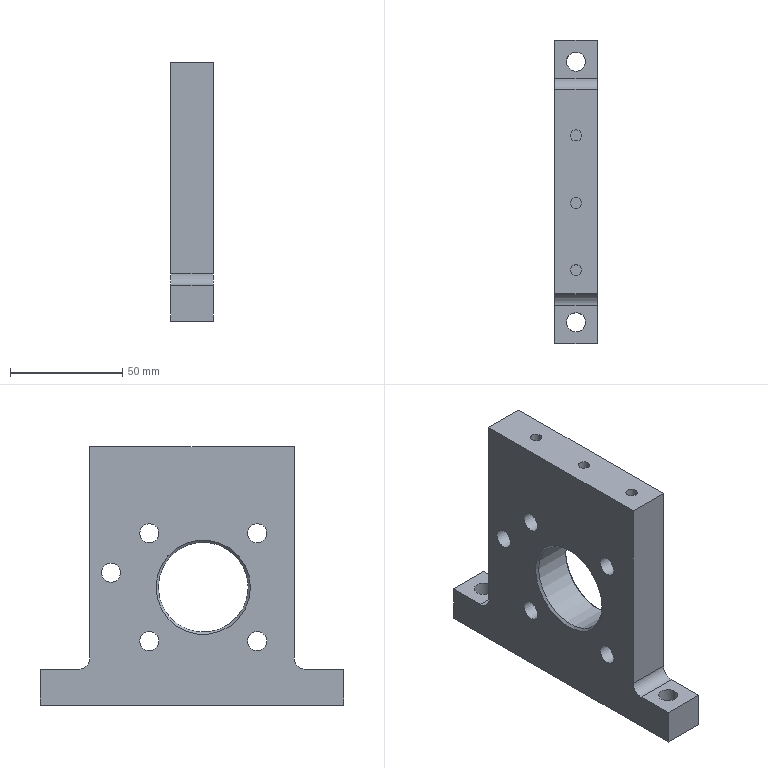Part | NX | 1 solid | 38 faces | box 19 x 135 x 115 mm | volume 176190 mm3 | cylinder 18 | plane 18 | cone 2 | commonest cylinder face diameters 8.5 x7 14 x5 5 x3 10 x2 40 x1
STEP:
#1=CARTESIAN_POINT('',(936.094,324.443,-201.3));
#2=VERTEX_POINT('',#1);
#3=CARTESIAN_POINT('',(936.094,317.443,-201.3));
#4=DIRECTION('',(-1.,0.,0.));
#5=DIRECTION('',(0.,1.,0.));
#6=AXIS2_PLACEMENT_3D('',#3,#4,#5);
#7=CIRCLE('',#6,7.);
#8=EDGE_CURVE('',#2,#2,#7,.T.);
#9=ORIENTED_EDGE('',*,*,#8,.F.);
#10=EDGE_LOOP('',(#9));
#11=FACE_BOUND('',#10,.T.);
#12=CARTESIAN_POINT('',(927.594,324.443,-201.3));
#13=VERTEX_POINT('',#12);
#14=CARTESIAN_POINT('',(927.594,317.443,-201.3));
#15=DIRECTION('',(-1.,0.,0.));
#16=DIRECTION('',(0.,1.,0.));
#17=AXIS2_PLACEMENT_3D('',#14,#15,#16);
#18=CIRCLE('',#17,7.);
#19=EDGE_CURVE('',#13,#13,#18,.T.);
#20=ORIENTED_EDGE('',*,*,#19,.T.);
#21=EDGE_LOOP('',(#20));
#22=FACE_BOUND('',#21,.T.);
#23=CARTESIAN_POINT('',(936.094,317.443,-201.3));
#24=DIRECTION('',(-1.,0.,0.));
#25=DIRECTION('',(0.,1.,0.));
#26=AXIS2_PLACEMENT_3D('',#23,#24,#25);
#27=CYLINDRICAL_SURFACE('',#26,7.);
#28=ADVANCED_FACE('',(#11,#22),#27,.F.);
#29=CARTESIAN_POINT('',(927.594,321.693,-201.3));
#30=VERTEX_POINT('',#29);
#31=CARTESIAN_POINT('',(927.594,317.443,-201.3));
#32=DIRECTION('',(1.,0.,0.));
#33=DIRECTION('',(0.,1.,0.));
#34=AXIS2_PLACEMENT_3D('',#31,#32,#33);
#35=CIRCLE('',#34,4.25);
#36=EDGE_CURVE('',#30,#30,#35,.T.);
#37=ORIENTED_EDGE('',*,*,#36,.F.);
#38=EDGE_LOOP('',(#37));
#39=FACE_BOUND('',#38,.T.);
#40=ORIENTED_EDGE('',*,*,#19,.F.);
#41=EDGE_LOOP('',(#40));
#42=FACE_BOUND('',#41,.T.);
#43=CARTESIAN_POINT('',(927.594,317.443,-201.3));
#44=DIRECTION('',(-1.,0.,0.));
#45=DIRECTION('',(0.,1.,0.));
#46=AXIS2_PLACEMENT_3D('',#43,#44,#45);
#47=PLANE('',#46);
#48=ADVANCED_FACE('',(#39,#42),#47,.F.);
#49=CARTESIAN_POINT('',(917.094,313.193,-201.3));
#50=VERTEX_POINT('',#49);
#51=CARTESIAN_POINT('',(917.094,317.443,-201.3));
#52=DIRECTION('',(1.,0.,0.));
#53=DIRECTION('',(0.,-1.,0.));
#54=AXIS2_PLACEMENT_3D('',#51,#52,#53);
#55=CIRCLE('',#54,4.25);
#56=EDGE_CURVE('',#50,#50,#55,.T.);
#57=ORIENTED_EDGE('',*,*,#56,.F.);
#58=EDGE_LOOP('',(#57));
#59=FACE_BOUND('',#58,.T.);
#60=ORIENTED_EDGE('',*,*,#36,.T.);
#61=EDGE_LOOP('',(#60));
#62=FACE_BOUND('',#61,.T.);
#63=CARTESIAN_POINT('',(917.094,317.443,-201.3));
#64=DIRECTION('',(1.,0.,0.));
#65=DIRECTION('',(0.,-1.,0.));
#66=AXIS2_PLACEMENT_3D('',#63,#64,#65);
#67=CYLINDRICAL_SURFACE('',#66,4.25);
#68=ADVANCED_FACE('',(#59,#62),#67,.F.);
#69=CARTESIAN_POINT('',(926.594,335.193,-260.3));
#70=VERTEX_POINT('',#69);
#71=CARTESIAN_POINT('',(926.594,339.443,-260.3));
#72=DIRECTION('',(0.,0.,1.));
#73=DIRECTION('',(0.,-1.,0.));
#74=AXIS2_PLACEMENT_3D('',#71,#72,#73);
#75=CIRCLE('',#74,4.25);
#76=EDGE_CURVE('',#70,#70,#75,.T.);
#77=ORIENTED_EDGE('',*,*,#76,.F.);
#78=EDGE_LOOP('',(#77));
#79=FACE_BOUND('',#78,.T.);
#80=CARTESIAN_POINT('',(930.844,339.443,-244.3));
#81=VERTEX_POINT('',#80);
#82=CARTESIAN_POINT('',(926.594,339.443,-244.3));
#83=DIRECTION('',(0.,0.,-1.));
#84=DIRECTION('',(1.,0.,0.));
#85=AXIS2_PLACEMENT_3D('',#82,#83,#84);
#86=CIRCLE('',#85,4.25);
#87=EDGE_CURVE('',#81,#81,#86,.T.);
#88=ORIENTED_EDGE('',*,*,#87,.F.);
#89=EDGE_LOOP('',(#88));
#90=FACE_BOUND('',#89,.T.);
#91=CARTESIAN_POINT('',(926.594,339.443,-244.3));
#92=DIRECTION('',(0.,0.,-1.));
#93=DIRECTION('',(-1.,0.,0.));
#94=AXIS2_PLACEMENT_3D('',#91,#92,#93);
#95=CYLINDRICAL_SURFACE('',#94,4.25);
#96=ADVANCED_FACE('',(#79,#90),#95,.F.);
#97=CARTESIAN_POINT('',(926.594,219.193,-260.3));
#98=VERTEX_POINT('',#97);
#99=CARTESIAN_POINT('',(926.594,223.443,-260.3));
#100=DIRECTION('',(0.,0.,1.));
#101=DIRECTION('',(0.,-1.,0.));
#102=AXIS2_PLACEMENT_3D('',#99,#100,#101);
#103=CIRCLE('',#102,4.25);
#104=EDGE_CURVE('',#98,#98,#103,.T.);
#105=ORIENTED_EDGE('',*,*,#104,.F.);
#106=EDGE_LOOP('',(#105));
#107=FACE_BOUND('',#106,.T.);
#108=CARTESIAN_POINT('',(922.344,223.443,-244.3));
#109=VERTEX_POINT('',#108);
#110=CARTESIAN_POINT('',(926.594,223.443,-244.3));
#111=DIRECTION('',(0.,0.,-1.));
#112=DIRECTION('',(-1.,0.,0.));
#113=AXIS2_PLACEMENT_3D('',#110,#111,#112);
#114=CIRCLE('',#113,4.25);
#115=EDGE_CURVE('',#109,#109,#114,.T.);
#116=ORIENTED_EDGE('',*,*,#115,.F.);
#117=EDGE_LOOP('',(#116));
#118=FACE_BOUND('',#117,.T.);
#119=CARTESIAN_POINT('',(926.594,223.443,-244.3));
#120=DIRECTION('',(0.,0.,-1.));
#121=DIRECTION('',(-1.,0.,0.));
#122=AXIS2_PLACEMENT_3D('',#119,#120,#121);
#123=CYLINDRICAL_SURFACE('',#122,4.25);
#124=ADVANCED_FACE('',(#107,#118),#123,.F.);
#125=CARTESIAN_POINT('',(924.094,276.443,-160.3));
#126=VERTEX_POINT('',#125);
#127=CARTESIAN_POINT('',(926.594,276.443,-160.3));
#128=DIRECTION('',(0.,0.,1.));
#129=DIRECTION('',(-1.,0.,0.));
#130=AXIS2_PLACEMENT_3D('',#127,#128,#129);
#131=CIRCLE('',#130,2.5);
#132=EDGE_CURVE('',#126,#126,#131,.T.);
#133=ORIENTED_EDGE('',*,*,#132,.T.);
#134=EDGE_LOOP('',(#133));
#135=FACE_BOUND('',#134,.T.);
#136=CARTESIAN_POINT('',(926.594,281.943,-160.3));
#137=DIRECTION('',(0.,0.,-1.));
#138=DIRECTION('',(0.,1.,0.));
#139=AXIS2_PLACEMENT_3D('',#136,#137,#138);
#140=PLANE('',#139);
#141=ADVANCED_FACE('',(#135),#140,.F.);
#142=ORIENTED_EDGE('',*,*,#132,.F.);
#143=EDGE_LOOP('',(#142));
#144=FACE_BOUND('',#143,.T.);
#145=CARTESIAN_POINT('',(924.094,276.443,-145.3));
#146=VERTEX_POINT('',#145);
#147=CARTESIAN_POINT('',(926.594,276.443,-145.3));
#148=DIRECTION('',(0.,0.,1.));
#149=DIRECTION('',(-1.,0.,0.));
#150=AXIS2_PLACEMENT_3D('',#147,#148,#149);
#151=CIRCLE('',#150,2.5);
#152=EDGE_CURVE('',#146,#146,#151,.T.);
#153=ORIENTED_EDGE('',*,*,#152,.T.);
#154=EDGE_LOOP('',(#153));
#155=FACE_BOUND('',#154,.T.);
#156=CARTESIAN_POINT('',(926.594,276.443,-145.3));
#157=DIRECTION('',(0.,0.,-1.));
#158=DIRECTION('',(-1.,0.,0.));
#159=AXIS2_PLACEMENT_3D('',#156,#157,#158);
#160=CYLINDRICAL_SURFACE('',#159,2.5);
#161=ADVANCED_FACE('',(#144,#155),#160,.F.);
#162=CARTESIAN_POINT('',(935.094,256.443,-207.8));
#163=VERTEX_POINT('',#162);
#164=CARTESIAN_POINT('',(935.094,276.443,-207.8));
#165=DIRECTION('',(1.,0.,0.));
#166=DIRECTION('',(0.,-1.,0.));
#167=AXIS2_PLACEMENT_3D('',#164,#165,#166);
#168=CIRCLE('',#167,20.);
#169=EDGE_CURVE('',#163,#163,#168,.T.);
#170=ORIENTED_EDGE('',*,*,#169,.F.);
#171=EDGE_LOOP('',(#170));
#172=FACE_BOUND('',#171,.T.);
#173=CARTESIAN_POINT('',(936.094,255.443,-207.8));
#174=VERTEX_POINT('',#173);
#175=CARTESIAN_POINT('',(936.094,276.443,-207.8));
#176=DIRECTION('',(-1.,0.,0.));
#177=DIRECTION('',(0.,-1.,0.));
#178=AXIS2_PLACEMENT_3D('',#175,#176,#177);
#179=CIRCLE('',#178,21.);
#180=EDGE_CURVE('',#174,#174,#179,.T.);
#181=ORIENTED_EDGE('',*,*,#180,.F.);
#182=EDGE_LOOP('',(#181));
#183=FACE_BOUND('',#182,.T.);
#184=CARTESIAN_POINT('',(935.094,276.443,-207.8));
#185=DIRECTION('',(1.,0.,0.));
#186=DIRECTION('',(0.,-1.,0.));
#187=AXIS2_PLACEMENT_3D('',#184,#185,#186);
#188=CONICAL_SURFACE('',#187,20.,0.7854);
#189=ADVANCED_FACE('',(#172,#183),#188,.F.);
#190=CARTESIAN_POINT('',(927.594,252.443,-227.55));
#191=VERTEX_POINT('',#190);
#192=CARTESIAN_POINT('',(927.594,252.443,-231.8));
#193=DIRECTION('',(-1.,0.,0.));
#194=DIRECTION('',(0.,0.,1.));
#195=AXIS2_PLACEMENT_3D('',#192,#193,#194);
#196=CIRCLE('',#195,4.25);
#197=EDGE_CURVE('',#191,#191,#196,.T.);
#198=ORIENTED_EDGE('',*,*,#197,.T.);
#199=EDGE_LOOP('',(#198));
#200=FACE_BOUND('',#199,.T.);
#201=CARTESIAN_POINT('',(927.594,252.443,-224.8));
#202=VERTEX_POINT('',#201);
#203=CARTESIAN_POINT('',(927.594,252.443,-231.8));
#204=DIRECTION('',(1.,0.,0.));
#205=DIRECTION('',(0.,0.,1.));
#206=AXIS2_PLACEMENT_3D('',#203,#204,#205);
#207=CIRCLE('',#206,7.);
#208=EDGE_CURVE('',#202,#202,#207,.T.);
#209=ORIENTED_EDGE('',*,*,#208,.T.);
#210=EDGE_LOOP('',(#209));
#211=FACE_BOUND('',#210,.T.);
#212=CARTESIAN_POINT('',(927.594,317.443,-201.3));
#213=DIRECTION('',(-1.,0.,0.));
#214=DIRECTION('',(0.,1.,0.));
#215=AXIS2_PLACEMENT_3D('',#212,#213,#214);
#216=PLANE('',#215);
#217=ADVANCED_FACE('',(#200,#211),#216,.F.);
#218=CARTESIAN_POINT('',(918.094,296.443,-207.8));
#219=VERTEX_POINT('',#218);
#220=CARTESIAN_POINT('',(918.094,276.443,-207.8));
#221=DIRECTION('',(-1.,0.,0.));
#222=DIRECTION('',(0.,1.,0.));
#223=AXIS2_PLACEMENT_3D('',#220,#221,#222);
#224=CIRCLE('',#223,20.);
#225=EDGE_CURVE('',#219,#219,#224,.T.);
#226=ORIENTED_EDGE('',*,*,#225,.F.);
#227=EDGE_LOOP('',(#226));
#228=FACE_BOUND('',#227,.T.);
#229=CARTESIAN_POINT('',(917.094,297.443,-207.8));
#230=VERTEX_POINT('',#229);
#231=CARTESIAN_POINT('',(917.094,276.443,-207.8));
#232=DIRECTION('',(1.,0.,0.));
#233=DIRECTION('',(0.,1.,0.));
#234=AXIS2_PLACEMENT_3D('',#231,#232,#233);
#235=CIRCLE('',#234,21.);
#236=EDGE_CURVE('',#230,#230,#235,.T.);
#237=ORIENTED_EDGE('',*,*,#236,.F.);
#238=EDGE_LOOP('',(#237));
#239=FACE_BOUND('',#238,.T.);
#240=CARTESIAN_POINT('',(918.094,276.443,-207.8));
#241=DIRECTION('',(-1.,0.,0.));
#242=DIRECTION('',(0.,1.,0.));
#243=AXIS2_PLACEMENT_3D('',#240,#241,#242);
#244=CONICAL_SURFACE('',#243,20.,0.7854);
#245=ADVANCED_FACE('',(#228,#239),#244,.F.);
#246=CARTESIAN_POINT('',(917.094,235.943,-239.3));
#247=VERTEX_POINT('',#246);
#248=CARTESIAN_POINT('',(917.094,235.943,-145.3));
#249=VERTEX_POINT('',#248);
#250=CARTESIAN_POINT('',(917.094,235.943,-204.8));
#251=DIRECTION('',(0.,0.,1.));
#252=VECTOR('',#251,1000.);
#253=LINE('',#250,#252);
#254=EDGE_CURVE('',#247,#249,#253,.T.);
#255=ORIENTED_EDGE('',*,*,#254,.T.);
#256=CARTESIAN_POINT('',(917.094,326.943,-145.3));
#257=VERTEX_POINT('',#256);
#258=CARTESIAN_POINT('',(917.094,329.943,-145.3));
#259=DIRECTION('',(0.,1.,0.));
#260=VECTOR('',#259,1000.);
#261=LINE('',#258,#260);
#262=EDGE_CURVE('',#249,#257,#261,.T.);
#263=ORIENTED_EDGE('',*,*,#262,.T.);
#264=CARTESIAN_POINT('',(917.094,326.943,-239.3));
#265=VERTEX_POINT('',#264);
#266=CARTESIAN_POINT('',(917.094,326.943,-204.8));
#267=DIRECTION('',(0.,0.,-1.));
#268=VECTOR('',#267,1000.);
#269=LINE('',#266,#268);
#270=EDGE_CURVE('',#257,#265,#269,.T.);
#271=ORIENTED_EDGE('',*,*,#270,.T.);
#272=CARTESIAN_POINT('',(917.094,331.943,-244.3));
#273=VERTEX_POINT('',#272);
#274=CARTESIAN_POINT('',(917.094,331.943,-239.3));
#275=DIRECTION('',(1.,0.,0.));
#276=DIRECTION('',(0.,1.,0.));
#277=AXIS2_PLACEMENT_3D('',#274,#275,#276);
#278=CIRCLE('',#277,5.);
#279=EDGE_CURVE('',#265,#273,#278,.T.);
#280=ORIENTED_EDGE('',*,*,#279,.T.);
#281=CARTESIAN_POINT('',(917.094,348.943,-244.3));
#282=VERTEX_POINT('',#281);
#283=CARTESIAN_POINT('',(917.094,329.943,-244.3));
#284=DIRECTION('',(0.,1.,0.));
#285=VECTOR('',#284,1000.);
#286=LINE('',#283,#285);
#287=EDGE_CURVE('',#273,#282,#286,.T.);
#288=ORIENTED_EDGE('',*,*,#287,.T.);
#289=CARTESIAN_POINT('',(917.094,348.943,-260.3));
#290=VERTEX_POINT('',#289);
#291=CARTESIAN_POINT('',(917.094,348.943,-204.8));
#292=DIRECTION('',(0.,0.,-1.));
#293=VECTOR('',#292,1000.);
#294=LINE('',#291,#293);
#295=EDGE_CURVE('',#282,#290,#294,.T.);
#296=ORIENTED_EDGE('',*,*,#295,.T.);
#297=CARTESIAN_POINT('',(917.094,213.943,-260.3));
#298=VERTEX_POINT('',#297);
#299=CARTESIAN_POINT('',(917.094,329.943,-260.3));
#300=DIRECTION('',(0.,1.,0.));
#301=VECTOR('',#300,1000.);
#302=LINE('',#299,#301);
#303=EDGE_CURVE('',#298,#290,#302,.T.);
#304=ORIENTED_EDGE('',*,*,#303,.F.);
#305=CARTESIAN_POINT('',(917.094,213.943,-244.3));
#306=VERTEX_POINT('',#305);
#307=CARTESIAN_POINT('',(917.094,213.943,-204.8));
#308=DIRECTION('',(0.,0.,1.));
#309=VECTOR('',#308,1000.);
#310=LINE('',#307,#309);
#311=EDGE_CURVE('',#298,#306,#310,.T.);
#312=ORIENTED_EDGE('',*,*,#311,.T.);
#313=CARTESIAN_POINT('',(917.094,230.943,-244.3));
#314=VERTEX_POINT('',#313);
#315=CARTESIAN_POINT('',(917.094,352.943,-244.3));
#316=DIRECTION('',(0.,1.,0.));
#317=VECTOR('',#316,1000.);
#318=LINE('',#315,#317);
#319=EDGE_CURVE('',#306,#314,#318,.T.);
#320=ORIENTED_EDGE('',*,*,#319,.T.);
#321=CARTESIAN_POINT('',(917.094,230.943,-239.3));
#322=DIRECTION('',(1.,0.,0.));
#323=DIRECTION('',(0.,1.,0.));
#324=AXIS2_PLACEMENT_3D('',#321,#322,#323);
#325=CIRCLE('',#324,5.);
#326=EDGE_CURVE('',#314,#247,#325,.T.);
#327=ORIENTED_EDGE('',*,*,#326,.T.);
#328=EDGE_LOOP('',(#255,#263,#271,#280,#288,#296,#304,#312,#320,#327));
#329=FACE_BOUND('',#328,.T.);
#330=ORIENTED_EDGE('',*,*,#236,.T.);
#331=EDGE_LOOP('',(#330));
#332=FACE_BOUND('',#331,.T.);
#333=CARTESIAN_POINT('',(917.094,252.443,-179.55));
#334=VERTEX_POINT('',#333);
#335=CARTESIAN_POINT('',(917.094,252.443,-183.8));
#336=DIRECTION('',(-1.,0.,0.));
#337=DIRECTION('',(0.,0.,1.));
#338=AXIS2_PLACEMENT_3D('',#335,#336,#337);
#339=CIRCLE('',#338,4.25);
#340=EDGE_CURVE('',#334,#334,#339,.T.);
#341=ORIENTED_EDGE('',*,*,#340,.F.);
#342=EDGE_LOOP('',(#341));
#343=FACE_BOUND('',#342,.T.);
#344=CARTESIAN_POINT('',(917.094,300.443,-179.55));
#345=VERTEX_POINT('',#344);
#346=CARTESIAN_POINT('',(917.094,300.443,-183.8));
#347=DIRECTION('',(-1.,0.,0.));
#348=DIRECTION('',(0.,0.,1.));
#349=AXIS2_PLACEMENT_3D('',#346,#347,#348);
#350=CIRCLE('',#349,4.25);
#351=EDGE_CURVE('',#345,#345,#350,.F.);
#352=ORIENTED_EDGE('',*,*,#351,.T.);
#353=EDGE_LOOP('',(#352));
#354=FACE_BOUND('',#353,.T.);
#355=CARTESIAN_POINT('',(917.094,252.443,-227.55));
#356=VERTEX_POINT('',#355);
#357=CARTESIAN_POINT('',(917.094,252.443,-231.8));
#358=DIRECTION('',(-1.,0.,0.));
#359=DIRECTION('',(0.,0.,1.));
#360=AXIS2_PLACEMENT_3D('',#357,#358,#359);
#361=CIRCLE('',#360,4.25);
#362=EDGE_CURVE('',#356,#356,#361,.F.);
#363=ORIENTED_EDGE('',*,*,#362,.T.);
#364=EDGE_LOOP('',(#363));
#365=FACE_BOUND('',#364,.T.);
#366=CARTESIAN_POINT('',(917.094,300.443,-227.55));
#367=VERTEX_POINT('',#366);
#368=CARTESIAN_POINT('',(917.094,300.443,-231.8));
#369=DIRECTION('',(-1.,0.,0.));
#370=DIRECTION('',(0.,0.,1.));
#371=AXIS2_PLACEMENT_3D('',#368,#369,#370);
#372=CIRCLE('',#371,4.25);
#373=EDGE_CURVE('',#367,#367,#372,.F.);
#374=ORIENTED_EDGE('',*,*,#373,.T.);
#375=EDGE_LOOP('',(#374));
#376=FACE_BOUND('',#375,.T.);
#377=ORIENTED_EDGE('',*,*,#56,.T.);
#378=EDGE_LOOP('',(#377));
#379=FACE_BOUND('',#378,.T.);
#380=CARTESIAN_POINT('',(917.094,329.943,-204.8));
#381=DIRECTION('',(-1.,0.,0.));
#382=DIRECTION('',(0.,1.,0.));
#383=AXIS2_PLACEMENT_3D('',#380,#381,#382);
#384=PLANE('',#383);
#385=ADVANCED_FACE('',(#329,#332,#343,#354,#365,#376,#379),#384,.T.);
#386=CARTESIAN_POINT('',(927.594,300.443,-227.55));
#387=VERTEX_POINT('',#386);
#388=CARTESIAN_POINT('',(927.594,300.443,-231.8));
#389=DIRECTION('',(-1.,0.,0.));
#390=DIRECTION('',(0.,0.,1.));
#391=AXIS2_PLACEMENT_3D('',#388,#389,#390);
#392=CIRCLE('',#391,4.25);
#393=EDGE_CURVE('',#387,#387,#392,.T.);
#394=ORIENTED_EDGE('',*,*,#393,.F.);
#395=EDGE_LOOP('',(#394));
#396=FACE_BOUND('',#395,.T.);
#397=ORIENTED_EDGE('',*,*,#373,.F.);
#398=EDGE_LOOP('',(#397));
#399=FACE_BOUND('',#398,.T.);
#400=CARTESIAN_POINT('',(917.094,300.443,-231.8));
#401=DIRECTION('',(1.,0.,0.));
#402=DIRECTION('',(0.,-1.,0.));
#403=AXIS2_PLACEMENT_3D('',#400,#401,#402);
#404=CYLINDRICAL_SURFACE('',#403,4.25);
#405=ADVANCED_FACE('',(#396,#399),#404,.F.);
#406=ORIENTED_EDGE('',*,*,#197,.F.);
#407=EDGE_LOOP('',(#406));
#408=FACE_BOUND('',#407,.T.);
#409=ORIENTED_EDGE('',*,*,#362,.F.);
#410=EDGE_LOOP('',(#409));
#411=FACE_BOUND('',#410,.T.);
#412=CARTESIAN_POINT('',(917.094,252.443,-231.8));
#413=DIRECTION('',(1.,0.,0.));
#414=DIRECTION('',(0.,-1.,0.));
#415=AXIS2_PLACEMENT_3D('',#412,#413,#414);
#416=CYLINDRICAL_SURFACE('',#415,4.25);
#417=ADVANCED_FACE('',(#408,#411),#416,.F.);
#418=CARTESIAN_POINT('',(927.594,300.443,-179.55));
#419=VERTEX_POINT('',#418);
#420=CARTESIAN_POINT('',(927.594,300.443,-183.8));
#421=DIRECTION('',(-1.,0.,0.));
#422=DIRECTION('',(0.,0.,1.));
#423=AXIS2_PLACEMENT_3D('',#420,#421,#422);
#424=CIRCLE('',#423,4.25);
#425=EDGE_CURVE('',#419,#419,#424,.F.);
#426=ORIENTED_EDGE('',*,*,#425,.T.);
#427=EDGE_LOOP('',(#426));
#428=FACE_BOUND('',#427,.T.);
#429=ORIENTED_EDGE('',*,*,#351,.F.);
#430=EDGE_LOOP('',(#429));
#431=FACE_BOUND('',#430,.T.);
#432=CARTESIAN_POINT('',(917.094,300.443,-183.8));
#433=DIRECTION('',(1.,0.,0.));
#434=DIRECTION('',(0.,-1.,0.));
#435=AXIS2_PLACEMENT_3D('',#432,#433,#434);
#436=CYLINDRICAL_SURFACE('',#435,4.25);
#437=ADVANCED_FACE('',(#428,#431),#436,.F.);
#438=CARTESIAN_POINT('',(927.594,252.443,-179.55));
#439=VERTEX_POINT('',#438);
#440=CARTESIAN_POINT('',(927.594,252.443,-183.8));
#441=DIRECTION('',(-1.,0.,0.));
#442=DIRECTION('',(0.,0.,1.));
#443=AXIS2_PLACEMENT_3D('',#440,#441,#442);
#444=CIRCLE('',#443,4.25);
#445=EDGE_CURVE('',#439,#439,#444,.F.);
#446=ORIENTED_EDGE('',*,*,#445,.T.);
#447=EDGE_LOOP('',(#446));
#448=FACE_BOUND('',#447,.T.);
#449=ORIENTED_EDGE('',*,*,#340,.T.);
#450=EDGE_LOOP('',(#449));
#451=FACE_BOUND('',#450,.T.);
#452=CARTESIAN_POINT('',(916.794,252.443,-183.8));
#453=DIRECTION('',(1.,0.,0.));
#454=DIRECTION('',(0.,-1.,0.));
#455=AXIS2_PLACEMENT_3D('',#452,#453,#454);
#456=CYLINDRICAL_SURFACE('',#455,4.25);
#457=ADVANCED_FACE('',(#448,#451),#456,.F.);
#458=CARTESIAN_POINT('',(927.594,252.443,-176.8));
#459=VERTEX_POINT('',#458);
#460=CARTESIAN_POINT('',(927.594,252.443,-183.8));
#461=DIRECTION('',(-1.,0.,0.));
#462=DIRECTION('',(0.,0.,1.));
#463=AXIS2_PLACEMENT_3D('',#460,#461,#462);
#464=CIRCLE('',#463,7.);
#465=EDGE_CURVE('',#459,#459,#464,.T.);
#466=ORIENTED_EDGE('',*,*,#465,.F.);
#467=EDGE_LOOP('',(#466));
#468=FACE_BOUND('',#467,.T.);
#469=ORIENTED_EDGE('',*,*,#445,.F.);
#470=EDGE_LOOP('',(#469));
#471=FACE_BOUND('',#470,.T.);
#472=CARTESIAN_POINT('',(927.594,317.443,-201.3));
#473=DIRECTION('',(-1.,0.,0.));
#474=DIRECTION('',(0.,1.,0.));
#475=AXIS2_PLACEMENT_3D('',#472,#473,#474);
#476=PLANE('',#475);
#477=ADVANCED_FACE('',(#468,#471),#476,.F.);
#478=ORIENTED_EDGE('',*,*,#393,.T.);
#479=EDGE_LOOP('',(#478));
#480=FACE_BOUND('',#479,.T.);
#481=CARTESIAN_POINT('',(927.594,300.443,-224.8));
#482=VERTEX_POINT('',#481);
#483=CARTESIAN_POINT('',(927.594,300.443,-231.8));
#484=DIRECTION('',(1.,0.,0.));
#485=DIRECTION('',(0.,0.,1.));
#486=AXIS2_PLACEMENT_3D('',#483,#484,#485);
#487=CIRCLE('',#486,7.);
#488=EDGE_CURVE('',#482,#482,#487,.T.);
#489=ORIENTED_EDGE('',*,*,#488,.T.);
#490=EDGE_LOOP('',(#489));
#491=FACE_BOUND('',#490,.T.);
#492=CARTESIAN_POINT('',(927.594,317.443,-201.3));
#493=DIRECTION('',(-1.,0.,0.));
#494=DIRECTION('',(0.,1.,0.));
#495=AXIS2_PLACEMENT_3D('',#492,#493,#494);
#496=PLANE('',#495);
#497=ADVANCED_FACE('',(#480,#491),#496,.F.);
#498=CARTESIAN_POINT('',(927.594,300.443,-176.8));
#499=VERTEX_POINT('',#498);
#500=CARTESIAN_POINT('',(927.594,300.443,-183.8));
#501=DIRECTION('',(-1.,0.,0.));
#502=DIRECTION('',(0.,0.,1.));
#503=AXIS2_PLACEMENT_3D('',#500,#501,#502);
#504=CIRCLE('',#503,7.);
#505=EDGE_CURVE('',#499,#499,#504,.T.);
#506=ORIENTED_EDGE('',*,*,#505,.F.);
#507=EDGE_LOOP('',(#506));
#508=FACE_BOUND('',#507,.T.);
#509=ORIENTED_EDGE('',*,*,#425,.F.);
#510=EDGE_LOOP('',(#509));
#511=FACE_BOUND('',#510,.T.);
#512=CARTESIAN_POINT('',(927.594,317.443,-201.3));
#513=DIRECTION('',(-1.,0.,0.));
#514=DIRECTION('',(0.,1.,0.));
#515=AXIS2_PLACEMENT_3D('',#512,#513,#514);
#516=PLANE('',#515);
#517=ADVANCED_FACE('',(#508,#511),#516,.F.);
#518=CARTESIAN_POINT('',(936.094,293.443,-231.8));
#519=VERTEX_POINT('',#518);
#520=CARTESIAN_POINT('',(936.094,300.443,-231.8));
#521=DIRECTION('',(1.,0.,0.));
#522=DIRECTION('',(0.,-1.,0.));
#523=AXIS2_PLACEMENT_3D('',#520,#521,#522);
#524=CIRCLE('',#523,7.);
#525=EDGE_CURVE('',#519,#519,#524,.T.);
#526=ORIENTED_EDGE('',*,*,#525,.T.);
#527=EDGE_LOOP('',(#526));
#528=FACE_BOUND('',#527,.T.);
#529=ORIENTED_EDGE('',*,*,#488,.F.);
#530=EDGE_LOOP('',(#529));
#531=FACE_BOUND('',#530,.T.);
#532=CARTESIAN_POINT('',(917.094,300.443,-231.8));
#533=DIRECTION('',(1.,0.,0.));
#534=DIRECTION('',(0.,-1.,0.));
#535=AXIS2_PLACEMENT_3D('',#532,#533,#534);
#536=CYLINDRICAL_SURFACE('',#535,7.);
#537=ADVANCED_FACE('',(#528,#531),#536,.F.);
#538=CARTESIAN_POINT('',(936.094,331.943,-244.3));
#539=VERTEX_POINT('',#538);
#540=CARTESIAN_POINT('',(936.094,348.943,-244.3));
#541=VERTEX_POINT('',#540);
#542=CARTESIAN_POINT('',(936.094,306.443,-244.3));
#543=DIRECTION('',(0.,1.,0.));
#544=VECTOR('',#543,1000.);
#545=LINE('',#542,#544);
#546=EDGE_CURVE('',#539,#541,#545,.T.);
#547=ORIENTED_EDGE('',*,*,#546,.F.);
#548=CARTESIAN_POINT('',(936.094,326.943,-239.3));
#549=VERTEX_POINT('',#548);
#550=CARTESIAN_POINT('',(936.094,331.943,-239.3));
#551=DIRECTION('',(-1.,0.,0.));
#552=DIRECTION('',(0.,-1.,0.));
#553=AXIS2_PLACEMENT_3D('',#550,#551,#552);
#554=CIRCLE('',#553,5.);
#555=EDGE_CURVE('',#539,#549,#554,.T.);
#556=ORIENTED_EDGE('',*,*,#555,.T.);
#557=CARTESIAN_POINT('',(936.094,326.943,-145.3));
#558=VERTEX_POINT('',#557);
#559=CARTESIAN_POINT('',(936.094,326.943,-209.8));
#560=DIRECTION('',(0.,0.,1.));
#561=VECTOR('',#560,1000.);
#562=LINE('',#559,#561);
#563=EDGE_CURVE('',#549,#558,#562,.T.);
#564=ORIENTED_EDGE('',*,*,#563,.T.);
#565=CARTESIAN_POINT('',(936.094,235.943,-145.3));
#566=VERTEX_POINT('',#565);
#567=CARTESIAN_POINT('',(936.094,276.493,-145.3));
#568=DIRECTION('',(0.,1.,0.));
#569=VECTOR('',#568,1000.);
#570=LINE('',#567,#569);
#571=EDGE_CURVE('',#566,#558,#570,.T.);
#572=ORIENTED_EDGE('',*,*,#571,.F.);
#573=CARTESIAN_POINT('',(936.094,235.943,-239.3));
#574=VERTEX_POINT('',#573);
#575=CARTESIAN_POINT('',(936.094,235.943,-209.8));
#576=DIRECTION('',(0.,0.,-1.));
#577=VECTOR('',#576,1000.);
#578=LINE('',#575,#577);
#579=EDGE_CURVE('',#566,#574,#578,.T.);
#580=ORIENTED_EDGE('',*,*,#579,.T.);
#581=CARTESIAN_POINT('',(936.094,230.943,-244.3));
#582=VERTEX_POINT('',#581);
#583=CARTESIAN_POINT('',(936.094,230.943,-239.3));
#584=DIRECTION('',(-1.,0.,0.));
#585=DIRECTION('',(0.,-1.,0.));
#586=AXIS2_PLACEMENT_3D('',#583,#584,#585);
#587=CIRCLE('',#586,5.);
#588=EDGE_CURVE('',#574,#582,#587,.T.);
#589=ORIENTED_EDGE('',*,*,#588,.T.);
#590=CARTESIAN_POINT('',(936.094,213.943,-244.3));
#591=VERTEX_POINT('',#590);
#592=CARTESIAN_POINT('',(936.094,306.443,-244.3));
#593=DIRECTION('',(0.,1.,0.));
#594=VECTOR('',#593,1000.);
#595=LINE('',#592,#594);
#596=EDGE_CURVE('',#591,#582,#595,.T.);
#597=ORIENTED_EDGE('',*,*,#596,.F.);
#598=CARTESIAN_POINT('',(936.094,213.943,-260.3));
#599=VERTEX_POINT('',#598);
#600=CARTESIAN_POINT('',(936.094,213.943,-209.8));
#601=DIRECTION('',(0.,0.,-1.));
#602=VECTOR('',#601,1000.);
#603=LINE('',#600,#602);
#604=EDGE_CURVE('',#591,#599,#603,.T.);
#605=ORIENTED_EDGE('',*,*,#604,.T.);
#606=CARTESIAN_POINT('',(936.094,348.943,-260.3));
#607=VERTEX_POINT('',#606);
#608=CARTESIAN_POINT('',(936.094,508.643,-260.3));
#609=DIRECTION('',(0.,1.,0.));
#610=VECTOR('',#609,1000.);
#611=LINE('',#608,#610);
#612=EDGE_CURVE('',#599,#607,#611,.T.);
#613=ORIENTED_EDGE('',*,*,#612,.T.);
#614=CARTESIAN_POINT('',(936.094,348.943,-209.8));
#615=DIRECTION('',(0.,0.,1.));
#616=VECTOR('',#615,1000.);
#617=LINE('',#614,#616);
#618=EDGE_CURVE('',#607,#541,#617,.T.);
#619=ORIENTED_EDGE('',*,*,#618,.T.);
#620=EDGE_LOOP('',(#547,#556,#564,#572,#580,#589,#597,#605,#613,#619));
#621=FACE_BOUND('',#620,.T.);
#622=CARTESIAN_POINT('',(936.094,245.443,-183.8));
#623=VERTEX_POINT('',#622);
#624=CARTESIAN_POINT('',(936.094,252.443,-183.8));
#625=DIRECTION('',(1.,0.,0.));
#626=DIRECTION('',(0.,-1.,0.));
#627=AXIS2_PLACEMENT_3D('',#624,#625,#626);
#628=CIRCLE('',#627,7.);
#629=EDGE_CURVE('',#623,#623,#628,.T.);
#630=ORIENTED_EDGE('',*,*,#629,.F.);
#631=EDGE_LOOP('',(#630));
#632=FACE_BOUND('',#631,.T.);
#633=CARTESIAN_POINT('',(936.094,293.443,-183.8));
#634=VERTEX_POINT('',#633);
#635=CARTESIAN_POINT('',(936.094,300.443,-183.8));
#636=DIRECTION('',(1.,0.,0.));
#637=DIRECTION('',(0.,-1.,0.));
#638=AXIS2_PLACEMENT_3D('',#635,#636,#637);
#639=CIRCLE('',#638,7.);
#640=EDGE_CURVE('',#634,#634,#639,.T.);
#641=ORIENTED_EDGE('',*,*,#640,.F.);
#642=EDGE_LOOP('',(#641));
#643=FACE_BOUND('',#642,.T.);
#644=CARTESIAN_POINT('',(936.094,245.443,-231.8));
#645=VERTEX_POINT('',#644);
#646=CARTESIAN_POINT('',(936.094,252.443,-231.8));
#647=DIRECTION('',(1.,0.,0.));
#648=DIRECTION('',(0.,-1.,0.));
#649=AXIS2_PLACEMENT_3D('',#646,#647,#648);
#650=CIRCLE('',#649,7.);
#651=EDGE_CURVE('',#645,#645,#650,.T.);
#652=ORIENTED_EDGE('',*,*,#651,.F.);
#653=EDGE_LOOP('',(#652));
#654=FACE_BOUND('',#653,.T.);
#655=ORIENTED_EDGE('',*,*,#525,.F.);
#656=EDGE_LOOP('',(#655));
#657=FACE_BOUND('',#656,.T.);
#658=ORIENTED_EDGE('',*,*,#180,.T.);
#659=EDGE_LOOP('',(#658));
#660=FACE_BOUND('',#659,.T.);
#661=ORIENTED_EDGE('',*,*,#8,.T.);
#662=EDGE_LOOP('',(#661));
#663=FACE_BOUND('',#662,.T.);
#664=CARTESIAN_POINT('',(936.094,272.943,-209.8));
#665=DIRECTION('',(1.,0.,0.));
#666=DIRECTION('',(0.,-1.,0.));
#667=AXIS2_PLACEMENT_3D('',#664,#665,#666);
#668=PLANE('',#667);
#669=ADVANCED_FACE('',(#621,#632,#643,#654,#657,#660,#663),#668,.T.);
#670=ORIENTED_EDGE('',*,*,#651,.T.);
#671=EDGE_LOOP('',(#670));
#672=FACE_BOUND('',#671,.T.);
#673=ORIENTED_EDGE('',*,*,#208,.F.);
#674=EDGE_LOOP('',(#673));
#675=FACE_BOUND('',#674,.T.);
#676=CARTESIAN_POINT('',(917.094,252.443,-231.8));
#677=DIRECTION('',(1.,0.,0.));
#678=DIRECTION('',(0.,-1.,0.));
#679=AXIS2_PLACEMENT_3D('',#676,#677,#678);
#680=CYLINDRICAL_SURFACE('',#679,7.);
#681=ADVANCED_FACE('',(#672,#675),#680,.F.);
#682=ORIENTED_EDGE('',*,*,#640,.T.);
#683=EDGE_LOOP('',(#682));
#684=FACE_BOUND('',#683,.T.);
#685=ORIENTED_EDGE('',*,*,#505,.T.);
#686=EDGE_LOOP('',(#685));
#687=FACE_BOUND('',#686,.T.);
#688=CARTESIAN_POINT('',(917.094,300.443,-183.8));
#689=DIRECTION('',(1.,0.,0.));
#690=DIRECTION('',(0.,-1.,0.));
#691=AXIS2_PLACEMENT_3D('',#688,#689,#690);
#692=CYLINDRICAL_SURFACE('',#691,7.);
#693=ADVANCED_FACE('',(#684,#687),#692,.F.);
#694=ORIENTED_EDGE('',*,*,#629,.T.);
#695=EDGE_LOOP('',(#694));
#696=FACE_BOUND('',#695,.T.);
#697=ORIENTED_EDGE('',*,*,#465,.T.);
#698=EDGE_LOOP('',(#697));
#699=FACE_BOUND('',#698,.T.);
#700=CARTESIAN_POINT('',(916.794,252.443,-183.8));
#701=DIRECTION('',(1.,0.,0.));
#702=DIRECTION('',(0.,-1.,0.));
#703=AXIS2_PLACEMENT_3D('',#700,#701,#702);
#704=CYLINDRICAL_SURFACE('',#703,7.);
#705=ADVANCED_FACE('',(#696,#699),#704,.F.);
#706=ORIENTED_EDGE('',*,*,#225,.T.);
#707=EDGE_LOOP('',(#706));
#708=FACE_BOUND('',#707,.T.);
#709=ORIENTED_EDGE('',*,*,#169,.T.);
#710=EDGE_LOOP('',(#709));
#711=FACE_BOUND('',#710,.T.);
#712=CARTESIAN_POINT('',(921.094,276.443,-207.8));
#713=DIRECTION('',(-1.,0.,0.));
#714=DIRECTION('',(0.,0.,1.));
#715=AXIS2_PLACEMENT_3D('',#712,#713,#714);
#716=CYLINDRICAL_SURFACE('',#715,20.);
#717=ADVANCED_FACE('',(#708,#711),#716,.F.);
#718=CARTESIAN_POINT('',(931.094,326.943,-239.3));
#719=DIRECTION('',(-1.,0.,0.));
#720=VECTOR('',#719,1000.);
#721=LINE('',#718,#720);
#722=EDGE_CURVE('',#549,#265,#721,.T.);
#723=ORIENTED_EDGE('',*,*,#722,.F.);
#724=ORIENTED_EDGE('',*,*,#555,.F.);
#725=CARTESIAN_POINT('',(918.594,331.943,-244.3));
#726=DIRECTION('',(1.,0.,0.));
#727=VECTOR('',#726,1000.);
#728=LINE('',#725,#727);
#729=EDGE_CURVE('',#273,#539,#728,.T.);
#730=ORIENTED_EDGE('',*,*,#729,.F.);
#731=ORIENTED_EDGE('',*,*,#279,.F.);
#732=EDGE_LOOP('',(#723,#724,#730,#731));
#733=FACE_BOUND('',#732,.T.);
#734=CARTESIAN_POINT('',(918.594,331.943,-239.3));
#735=DIRECTION('',(1.,0.,0.));
#736=DIRECTION('',(0.,-1.,0.));
#737=AXIS2_PLACEMENT_3D('',#734,#735,#736);
#738=CYLINDRICAL_SURFACE('',#737,5.);
#739=ADVANCED_FACE('',(#733),#738,.F.);
#740=CARTESIAN_POINT('',(931.094,230.943,-244.3));
#741=DIRECTION('',(-1.,0.,0.));
#742=VECTOR('',#741,1000.);
#743=LINE('',#740,#742);
#744=EDGE_CURVE('',#582,#314,#743,.T.);
#745=ORIENTED_EDGE('',*,*,#744,.F.);
#746=ORIENTED_EDGE('',*,*,#588,.F.);
#747=CARTESIAN_POINT('',(917.094,235.943,-239.3));
#748=DIRECTION('',(1.,0.,0.));
#749=VECTOR('',#748,1000.);
#750=LINE('',#747,#749);
#751=EDGE_CURVE('',#247,#574,#750,.T.);
#752=ORIENTED_EDGE('',*,*,#751,.F.);
#753=ORIENTED_EDGE('',*,*,#326,.F.);
#754=EDGE_LOOP('',(#745,#746,#752,#753));
#755=FACE_BOUND('',#754,.T.);
#756=CARTESIAN_POINT('',(918.594,230.943,-239.3));
#757=DIRECTION('',(-1.,0.,0.));
#758=DIRECTION('',(0.,1.,0.));
#759=AXIS2_PLACEMENT_3D('',#756,#757,#758);
#760=CYLINDRICAL_SURFACE('',#759,5.);
#761=ADVANCED_FACE('',(#755),#760,.F.);
#762=ORIENTED_EDGE('',*,*,#319,.F.);
#763=CARTESIAN_POINT('',(917.094,213.943,-244.3));
#764=DIRECTION('',(-1.,0.,0.));
#765=VECTOR('',#764,1000.);
#766=LINE('',#763,#765);
#767=EDGE_CURVE('',#591,#306,#766,.T.);
#768=ORIENTED_EDGE('',*,*,#767,.F.);
#769=ORIENTED_EDGE('',*,*,#596,.T.);
#770=ORIENTED_EDGE('',*,*,#744,.T.);
#771=EDGE_LOOP('',(#762,#768,#769,#770));
#772=FACE_BOUND('',#771,.T.);
#773=ORIENTED_EDGE('',*,*,#115,.T.);
#774=EDGE_LOOP('',(#773));
#775=FACE_BOUND('',#774,.T.);
#776=CARTESIAN_POINT('',(918.594,306.443,-244.3));
#777=DIRECTION('',(0.,0.,1.));
#778=DIRECTION('',(0.,-1.,0.));
#779=AXIS2_PLACEMENT_3D('',#776,#777,#778);
#780=PLANE('',#779);
#781=ADVANCED_FACE('',(#772,#775),#780,.T.);
#782=CARTESIAN_POINT('',(917.094,213.943,-260.3));
#783=DIRECTION('',(-1.,0.,0.));
#784=VECTOR('',#783,1000.);
#785=LINE('',#782,#784);
#786=EDGE_CURVE('',#599,#298,#785,.T.);
#787=ORIENTED_EDGE('',*,*,#786,.F.);
#788=ORIENTED_EDGE('',*,*,#604,.F.);
#789=ORIENTED_EDGE('',*,*,#767,.T.);
#790=ORIENTED_EDGE('',*,*,#311,.F.);
#791=EDGE_LOOP('',(#787,#788,#789,#790));
#792=FACE_BOUND('',#791,.T.);
#793=CARTESIAN_POINT('',(917.094,213.943,-204.8));
#794=DIRECTION('',(0.,-1.,0.));
#795=DIRECTION('',(-1.,0.,0.));
#796=AXIS2_PLACEMENT_3D('',#793,#794,#795);
#797=PLANE('',#796);
#798=ADVANCED_FACE('',(#792),#797,.T.);
#799=CARTESIAN_POINT('',(917.094,348.943,-244.3));
#800=DIRECTION('',(1.,0.,0.));
#801=VECTOR('',#800,1000.);
#802=LINE('',#799,#801);
#803=EDGE_CURVE('',#282,#541,#802,.T.);
#804=ORIENTED_EDGE('',*,*,#803,.T.);
#805=ORIENTED_EDGE('',*,*,#618,.F.);
#806=CARTESIAN_POINT('',(917.094,348.943,-260.3));
#807=DIRECTION('',(1.,0.,0.));
#808=VECTOR('',#807,1000.);
#809=LINE('',#806,#808);
#810=EDGE_CURVE('',#290,#607,#809,.T.);
#811=ORIENTED_EDGE('',*,*,#810,.F.);
#812=ORIENTED_EDGE('',*,*,#295,.F.);
#813=EDGE_LOOP('',(#804,#805,#811,#812));
#814=FACE_BOUND('',#813,.T.);
#815=CARTESIAN_POINT('',(917.094,348.943,-204.8));
#816=DIRECTION('',(0.,1.,0.));
#817=DIRECTION('',(1.,0.,0.));
#818=AXIS2_PLACEMENT_3D('',#815,#816,#817);
#819=PLANE('',#818);
#820=ADVANCED_FACE('',(#814),#819,.T.);
#821=ORIENTED_EDGE('',*,*,#810,.T.);
#822=ORIENTED_EDGE('',*,*,#612,.F.);
#823=ORIENTED_EDGE('',*,*,#786,.T.);
#824=ORIENTED_EDGE('',*,*,#303,.T.);
#825=EDGE_LOOP('',(#821,#822,#823,#824));
#826=FACE_BOUND('',#825,.T.);
#827=ORIENTED_EDGE('',*,*,#104,.T.);
#828=EDGE_LOOP('',(#827));
#829=FACE_BOUND('',#828,.T.);
#830=ORIENTED_EDGE('',*,*,#76,.T.);
#831=EDGE_LOOP('',(#830));
#832=FACE_BOUND('',#831,.T.);
#833=CARTESIAN_POINT('',(784.166,508.643,-260.3));
#834=DIRECTION('',(0.,0.,1.));
#835=DIRECTION('',(0.,-1.,0.));
#836=AXIS2_PLACEMENT_3D('',#833,#834,#835);
#837=PLANE('',#836);
#838=ADVANCED_FACE('',(#826,#829,#832),#837,.F.);
#839=ORIENTED_EDGE('',*,*,#287,.F.);
#840=ORIENTED_EDGE('',*,*,#729,.T.);
#841=ORIENTED_EDGE('',*,*,#546,.T.);
#842=ORIENTED_EDGE('',*,*,#803,.F.);
#843=EDGE_LOOP('',(#839,#840,#841,#842));
#844=FACE_BOUND('',#843,.T.);
#845=ORIENTED_EDGE('',*,*,#87,.T.);
#846=EDGE_LOOP('',(#845));
#847=FACE_BOUND('',#846,.T.);
#848=CARTESIAN_POINT('',(918.594,306.443,-244.3));
#849=DIRECTION('',(0.,0.,1.));
#850=DIRECTION('',(0.,-1.,0.));
#851=AXIS2_PLACEMENT_3D('',#848,#849,#850);
#852=PLANE('',#851);
#853=ADVANCED_FACE('',(#844,#847),#852,.T.);
#854=ORIENTED_EDGE('',*,*,#751,.T.);
#855=ORIENTED_EDGE('',*,*,#579,.F.);
#856=CARTESIAN_POINT('',(917.094,235.943,-145.3));
#857=DIRECTION('',(-1.,0.,0.));
#858=VECTOR('',#857,1000.);
#859=LINE('',#856,#858);
#860=EDGE_CURVE('',#566,#249,#859,.T.);
#861=ORIENTED_EDGE('',*,*,#860,.T.);
#862=ORIENTED_EDGE('',*,*,#254,.F.);
#863=EDGE_LOOP('',(#854,#855,#861,#862));
#864=FACE_BOUND('',#863,.T.);
#865=CARTESIAN_POINT('',(917.094,235.943,-204.8));
#866=DIRECTION('',(0.,-1.,0.));
#867=DIRECTION('',(-1.,0.,0.));
#868=AXIS2_PLACEMENT_3D('',#865,#866,#867);
#869=PLANE('',#868);
#870=ADVANCED_FACE('',(#864),#869,.T.);
#871=ORIENTED_EDGE('',*,*,#152,.F.);
#872=EDGE_LOOP('',(#871));
#873=FACE_BOUND('',#872,.T.);
#874=CARTESIAN_POINT('',(924.094,246.443,-145.3));
#875=VERTEX_POINT('',#874);
#876=CARTESIAN_POINT('',(926.594,246.443,-145.3));
#877=DIRECTION('',(0.,0.,-1.));
#878=DIRECTION('',(-1.,0.,0.));
#879=AXIS2_PLACEMENT_3D('',#876,#877,#878);
#880=CIRCLE('',#879,2.5);
#881=EDGE_CURVE('',#875,#875,#880,.T.);
#882=ORIENTED_EDGE('',*,*,#881,.T.);
#883=EDGE_LOOP('',(#882));
#884=FACE_BOUND('',#883,.T.);
#885=ORIENTED_EDGE('',*,*,#860,.F.);
#886=ORIENTED_EDGE('',*,*,#571,.T.);
#887=CARTESIAN_POINT('',(917.094,326.943,-145.3));
#888=DIRECTION('',(1.,0.,0.));
#889=VECTOR('',#888,1000.);
#890=LINE('',#887,#889);
#891=EDGE_CURVE('',#257,#558,#890,.T.);
#892=ORIENTED_EDGE('',*,*,#891,.F.);
#893=ORIENTED_EDGE('',*,*,#262,.F.);
#894=EDGE_LOOP('',(#885,#886,#892,#893));
#895=FACE_BOUND('',#894,.T.);
#896=CARTESIAN_POINT('',(924.094,306.443,-145.3));
#897=VERTEX_POINT('',#896);
#898=CARTESIAN_POINT('',(926.594,306.443,-145.3));
#899=DIRECTION('',(0.,0.,-1.));
#900=DIRECTION('',(-1.,0.,0.));
#901=AXIS2_PLACEMENT_3D('',#898,#899,#900);
#902=CIRCLE('',#901,2.5);
#903=EDGE_CURVE('',#897,#897,#902,.T.);
#904=ORIENTED_EDGE('',*,*,#903,.T.);
#905=EDGE_LOOP('',(#904));
#906=FACE_BOUND('',#905,.T.);
#907=CARTESIAN_POINT('',(855.194,276.493,-145.3));
#908=DIRECTION('',(0.,0.,-1.));
#909=DIRECTION('',(1.,0.,0.));
#910=AXIS2_PLACEMENT_3D('',#907,#908,#909);
#911=PLANE('',#910);
#912=ADVANCED_FACE('',(#873,#884,#895,#906),#911,.F.);
#913=ORIENTED_EDGE('',*,*,#891,.T.);
#914=ORIENTED_EDGE('',*,*,#563,.F.);
#915=ORIENTED_EDGE('',*,*,#722,.T.);
#916=ORIENTED_EDGE('',*,*,#270,.F.);
#917=EDGE_LOOP('',(#913,#914,#915,#916));
#918=FACE_BOUND('',#917,.T.);
#919=CARTESIAN_POINT('',(917.094,326.943,-204.8));
#920=DIRECTION('',(0.,1.,0.));
#921=DIRECTION('',(1.,0.,0.));
#922=AXIS2_PLACEMENT_3D('',#919,#920,#921);
#923=PLANE('',#922);
#924=ADVANCED_FACE('',(#918),#923,.T.);
#925=CARTESIAN_POINT('',(924.094,246.443,-160.3));
#926=VERTEX_POINT('',#925);
#927=CARTESIAN_POINT('',(926.594,246.443,-160.3));
#928=DIRECTION('',(0.,0.,-1.));
#929=DIRECTION('',(-1.,0.,0.));
#930=AXIS2_PLACEMENT_3D('',#927,#928,#929);
#931=CIRCLE('',#930,2.5);
#932=EDGE_CURVE('',#926,#926,#931,.T.);
#933=ORIENTED_EDGE('',*,*,#932,.F.);
#934=EDGE_LOOP('',(#933));
#935=FACE_BOUND('',#934,.T.);
#936=CARTESIAN_POINT('',(926.594,281.943,-160.3));
#937=DIRECTION('',(0.,0.,-1.));
#938=DIRECTION('',(0.,1.,0.));
#939=AXIS2_PLACEMENT_3D('',#936,#937,#938);
#940=PLANE('',#939);
#941=ADVANCED_FACE('',(#935),#940,.F.);
#942=ORIENTED_EDGE('',*,*,#932,.T.);
#943=EDGE_LOOP('',(#942));
#944=FACE_BOUND('',#943,.T.);
#945=ORIENTED_EDGE('',*,*,#881,.F.);
#946=EDGE_LOOP('',(#945));
#947=FACE_BOUND('',#946,.T.);
#948=CARTESIAN_POINT('',(926.594,246.443,-145.3));
#949=DIRECTION('',(0.,0.,-1.));
#950=DIRECTION('',(-1.,0.,0.));
#951=AXIS2_PLACEMENT_3D('',#948,#949,#950);
#952=CYLINDRICAL_SURFACE('',#951,2.5);
#953=ADVANCED_FACE('',(#944,#947),#952,.F.);
#954=CARTESIAN_POINT('',(924.094,306.443,-160.3));
#955=VERTEX_POINT('',#954);
#956=CARTESIAN_POINT('',(926.594,306.443,-160.3));
#957=DIRECTION('',(0.,0.,-1.));
#958=DIRECTION('',(-1.,0.,0.));
#959=AXIS2_PLACEMENT_3D('',#956,#957,#958);
#960=CIRCLE('',#959,2.5);
#961=EDGE_CURVE('',#955,#955,#960,.T.);
#962=ORIENTED_EDGE('',*,*,#961,.F.);
#963=EDGE_LOOP('',(#962));
#964=FACE_BOUND('',#963,.T.);
#965=CARTESIAN_POINT('',(926.594,281.943,-160.3));
#966=DIRECTION('',(0.,0.,-1.));
#967=DIRECTION('',(0.,1.,0.));
#968=AXIS2_PLACEMENT_3D('',#965,#966,#967);
#969=PLANE('',#968);
#970=ADVANCED_FACE('',(#964),#969,.F.);
#971=ORIENTED_EDGE('',*,*,#961,.T.);
#972=EDGE_LOOP('',(#971));
#973=FACE_BOUND('',#972,.T.);
#974=ORIENTED_EDGE('',*,*,#903,.F.);
#975=EDGE_LOOP('',(#974));
#976=FACE_BOUND('',#975,.T.);
#977=CARTESIAN_POINT('',(926.594,306.443,-145.3));
#978=DIRECTION('',(0.,0.,-1.));
#979=DIRECTION('',(-1.,0.,0.));
#980=AXIS2_PLACEMENT_3D('',#977,#978,#979);
#981=CYLINDRICAL_SURFACE('',#980,2.5);
#982=ADVANCED_FACE('',(#973,#976),#981,.F.);
#983=CLOSED_SHELL('',(#28,#48,#68,#96,#124,#141,#161,#189,#217,#245,#385,#405,#417,#437,#457,#477,#497,#517,#537,#669,#681,#693,#705,#717,#739,#761,#781,#798,#820,#838,#853,#870,#912,#924,#941,#953,#970,#982));
#984=MANIFOLD_SOLID_BREP('',#983);
#985=(LENGTH_UNIT()NAMED_UNIT(*)SI_UNIT(.MILLI.,.METRE.));
#986=UNCERTAINTY_MEASURE_WITH_UNIT(LENGTH_MEASURE(0.00001),#985,'','');
#987=(NAMED_UNIT(*)PLANE_ANGLE_UNIT()SI_UNIT($,.RADIAN.));
#988=(NAMED_UNIT(*)SI_UNIT($,.STERADIAN.)SOLID_ANGLE_UNIT());
#989=(GEOMETRIC_REPRESENTATION_CONTEXT(3)GLOBAL_UNCERTAINTY_ASSIGNED_CONTEXT((#986))GLOBAL_UNIT_ASSIGNED_CONTEXT((#985,#987,#988))REPRESENTATION_CONTEXT('',''));
#990=ADVANCED_BREP_SHAPE_REPRESENTATION('',(#984),#989);